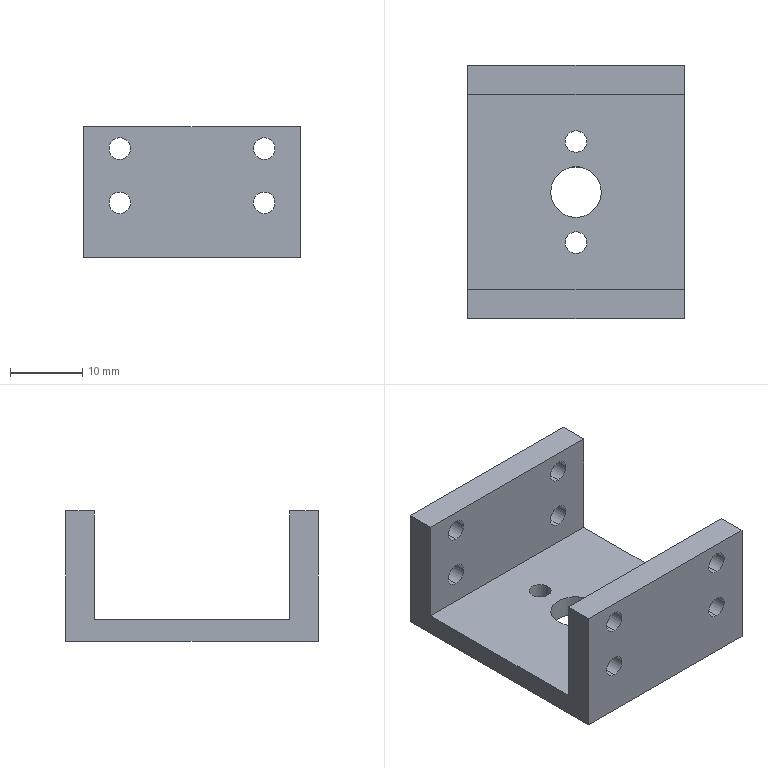Part | SolidWorks | features ICE 2, Extrusion 1, MirrorPattern 1 | 1 solid | 32 faces | box 30 x 35 x 18 mm | volume 6366 mm3 | cylinder 22 | plane 10 | commonest cylinder face diameters 3 x20 7 x2
STEP:
#1=CARTESIAN_POINT('',(-10.,-17.5,9.));
#2=VERTEX_POINT('',#1);
#3=CARTESIAN_POINT('',(-10.,-17.5,6.));
#4=VERTEX_POINT('',#3);
#5=CARTESIAN_POINT('',(-10.,-17.5,7.5));
#6=DIRECTION('',(0.,-1.,0.));
#7=DIRECTION('',(0.,0.,1.));
#8=AXIS2_PLACEMENT_3D('',#5,#6,#7);
#9=CIRCLE('',#8,1.5);
#10=EDGE_CURVE('',#2,#4,#9,.T.);
#11=ORIENTED_EDGE('',*,*,#10,.T.);
#12=CARTESIAN_POINT('',(-10.,-13.5,6.));
#13=VERTEX_POINT('',#12);
#14=CARTESIAN_POINT('',(-10.,-28.5,6.));
#15=DIRECTION('',(0.,1.,0.));
#16=VECTOR('',#15,1000.);
#17=LINE('',#14,#16);
#18=EDGE_CURVE('',#4,#13,#17,.T.);
#19=ORIENTED_EDGE('',*,*,#18,.T.);
#20=CARTESIAN_POINT('',(-10.,-13.5,9.));
#21=VERTEX_POINT('',#20);
#22=CARTESIAN_POINT('',(-10.,-13.5,7.5));
#23=DIRECTION('',(0.,-1.,0.));
#24=DIRECTION('',(0.,0.,1.));
#25=AXIS2_PLACEMENT_3D('',#22,#23,#24);
#26=CIRCLE('',#25,1.5);
#27=EDGE_CURVE('',#21,#13,#26,.T.);
#28=ORIENTED_EDGE('',*,*,#27,.F.);
#29=CARTESIAN_POINT('',(-10.,-28.5,9.));
#30=DIRECTION('',(0.,1.,0.));
#31=VECTOR('',#30,1000.);
#32=LINE('',#29,#31);
#33=EDGE_CURVE('',#2,#21,#32,.T.);
#34=ORIENTED_EDGE('',*,*,#33,.F.);
#35=EDGE_LOOP('',(#11,#19,#28,#34));
#36=FACE_OUTER_BOUND('',#35,.T.);
#37=CARTESIAN_POINT('',(-10.,-28.5,7.5));
#38=DIRECTION('',(0.,1.,0.));
#39=DIRECTION('',(0.,0.,1.));
#40=AXIS2_PLACEMENT_3D('',#37,#38,#39);
#41=CYLINDRICAL_SURFACE('',#40,1.5);
#42=ADVANCED_FACE('',(#36),#41,.F.);
#43=CARTESIAN_POINT('',(10.,-17.5,9.));
#44=VERTEX_POINT('',#43);
#45=CARTESIAN_POINT('',(10.,-17.5,6.));
#46=VERTEX_POINT('',#45);
#47=CARTESIAN_POINT('',(10.,-17.5,7.5));
#48=DIRECTION('',(0.,-1.,0.));
#49=DIRECTION('',(0.,0.,1.));
#50=AXIS2_PLACEMENT_3D('',#47,#48,#49);
#51=CIRCLE('',#50,1.5);
#52=EDGE_CURVE('',#44,#46,#51,.T.);
#53=ORIENTED_EDGE('',*,*,#52,.T.);
#54=CARTESIAN_POINT('',(10.,-13.5,6.));
#55=VERTEX_POINT('',#54);
#56=CARTESIAN_POINT('',(10.,-28.5,6.));
#57=DIRECTION('',(0.,1.,0.));
#58=VECTOR('',#57,1000.);
#59=LINE('',#56,#58);
#60=EDGE_CURVE('',#46,#55,#59,.T.);
#61=ORIENTED_EDGE('',*,*,#60,.T.);
#62=CARTESIAN_POINT('',(10.,-13.5,9.));
#63=VERTEX_POINT('',#62);
#64=CARTESIAN_POINT('',(10.,-13.5,7.5));
#65=DIRECTION('',(0.,-1.,0.));
#66=DIRECTION('',(0.,0.,-1.));
#67=AXIS2_PLACEMENT_3D('',#64,#65,#66);
#68=CIRCLE('',#67,1.5);
#69=EDGE_CURVE('',#63,#55,#68,.T.);
#70=ORIENTED_EDGE('',*,*,#69,.F.);
#71=CARTESIAN_POINT('',(10.,-28.5,9.));
#72=DIRECTION('',(0.,1.,0.));
#73=VECTOR('',#72,1000.);
#74=LINE('',#71,#73);
#75=EDGE_CURVE('',#44,#63,#74,.T.);
#76=ORIENTED_EDGE('',*,*,#75,.F.);
#77=EDGE_LOOP('',(#53,#61,#70,#76));
#78=FACE_OUTER_BOUND('',#77,.T.);
#79=CARTESIAN_POINT('',(10.,-28.5,7.5));
#80=DIRECTION('',(0.,1.,0.));
#81=DIRECTION('',(0.,0.,1.));
#82=AXIS2_PLACEMENT_3D('',#79,#80,#81);
#83=CYLINDRICAL_SURFACE('',#82,1.5);
#84=ADVANCED_FACE('',(#78),#83,.F.);
#85=CARTESIAN_POINT('',(10.,-17.5,16.5));
#86=VERTEX_POINT('',#85);
#87=CARTESIAN_POINT('',(10.,-17.5,13.5));
#88=VERTEX_POINT('',#87);
#89=CARTESIAN_POINT('',(10.,-17.5,15.));
#90=DIRECTION('',(0.,-1.,0.));
#91=DIRECTION('',(0.,0.,1.));
#92=AXIS2_PLACEMENT_3D('',#89,#90,#91);
#93=CIRCLE('',#92,1.5);
#94=EDGE_CURVE('',#86,#88,#93,.T.);
#95=ORIENTED_EDGE('',*,*,#94,.T.);
#96=CARTESIAN_POINT('',(10.,-13.5,13.5));
#97=VERTEX_POINT('',#96);
#98=CARTESIAN_POINT('',(10.,-28.5,13.5));
#99=DIRECTION('',(0.,1.,0.));
#100=VECTOR('',#99,1000.);
#101=LINE('',#98,#100);
#102=EDGE_CURVE('',#88,#97,#101,.T.);
#103=ORIENTED_EDGE('',*,*,#102,.T.);
#104=CARTESIAN_POINT('',(10.,-13.5,16.5));
#105=VERTEX_POINT('',#104);
#106=CARTESIAN_POINT('',(10.,-13.5,15.));
#107=DIRECTION('',(0.,-1.,0.));
#108=DIRECTION('',(0.,0.,1.));
#109=AXIS2_PLACEMENT_3D('',#106,#107,#108);
#110=CIRCLE('',#109,1.5);
#111=EDGE_CURVE('',#105,#97,#110,.T.);
#112=ORIENTED_EDGE('',*,*,#111,.F.);
#113=CARTESIAN_POINT('',(10.,-28.5,16.5));
#114=DIRECTION('',(0.,1.,0.));
#115=VECTOR('',#114,1000.);
#116=LINE('',#113,#115);
#117=EDGE_CURVE('',#86,#105,#116,.T.);
#118=ORIENTED_EDGE('',*,*,#117,.F.);
#119=EDGE_LOOP('',(#95,#103,#112,#118));
#120=FACE_OUTER_BOUND('',#119,.T.);
#121=CARTESIAN_POINT('',(10.,-28.5,15.));
#122=DIRECTION('',(0.,1.,0.));
#123=DIRECTION('',(0.,0.,1.));
#124=AXIS2_PLACEMENT_3D('',#121,#122,#123);
#125=CYLINDRICAL_SURFACE('',#124,1.5);
#126=ADVANCED_FACE('',(#120),#125,.F.);
#127=CARTESIAN_POINT('',(-10.,-17.5,16.5));
#128=VERTEX_POINT('',#127);
#129=CARTESIAN_POINT('',(-10.,-17.5,13.5));
#130=VERTEX_POINT('',#129);
#131=CARTESIAN_POINT('',(-10.,-17.5,15.));
#132=DIRECTION('',(0.,-1.,0.));
#133=DIRECTION('',(0.,0.,1.));
#134=AXIS2_PLACEMENT_3D('',#131,#132,#133);
#135=CIRCLE('',#134,1.5);
#136=EDGE_CURVE('',#128,#130,#135,.T.);
#137=ORIENTED_EDGE('',*,*,#136,.T.);
#138=CARTESIAN_POINT('',(-10.,-13.5,13.5));
#139=VERTEX_POINT('',#138);
#140=CARTESIAN_POINT('',(-10.,-28.5,13.5));
#141=DIRECTION('',(0.,1.,0.));
#142=VECTOR('',#141,1000.);
#143=LINE('',#140,#142);
#144=EDGE_CURVE('',#130,#139,#143,.T.);
#145=ORIENTED_EDGE('',*,*,#144,.T.);
#146=CARTESIAN_POINT('',(-10.,-13.5,16.5));
#147=VERTEX_POINT('',#146);
#148=CARTESIAN_POINT('',(-10.,-13.5,15.));
#149=DIRECTION('',(0.,-1.,0.));
#150=DIRECTION('',(0.,0.,-1.));
#151=AXIS2_PLACEMENT_3D('',#148,#149,#150);
#152=CIRCLE('',#151,1.5);
#153=EDGE_CURVE('',#147,#139,#152,.T.);
#154=ORIENTED_EDGE('',*,*,#153,.F.);
#155=CARTESIAN_POINT('',(-10.,-28.5,16.5));
#156=DIRECTION('',(0.,1.,0.));
#157=VECTOR('',#156,1000.);
#158=LINE('',#155,#157);
#159=EDGE_CURVE('',#128,#147,#158,.T.);
#160=ORIENTED_EDGE('',*,*,#159,.F.);
#161=EDGE_LOOP('',(#137,#145,#154,#160));
#162=FACE_OUTER_BOUND('',#161,.T.);
#163=CARTESIAN_POINT('',(-10.,-28.5,15.));
#164=DIRECTION('',(0.,1.,0.));
#165=DIRECTION('',(0.,0.,1.));
#166=AXIS2_PLACEMENT_3D('',#163,#164,#165);
#167=CYLINDRICAL_SURFACE('',#166,1.5);
#168=ADVANCED_FACE('',(#162),#167,.F.);
#169=CARTESIAN_POINT('',(-10.,17.5,9.));
#170=VERTEX_POINT('',#169);
#171=CARTESIAN_POINT('',(-10.,17.5,6.));
#172=VERTEX_POINT('',#171);
#173=CARTESIAN_POINT('',(-10.,17.5,7.5));
#174=DIRECTION('',(0.,-1.,0.));
#175=DIRECTION('',(0.,0.,-1.));
#176=AXIS2_PLACEMENT_3D('',#173,#174,#175);
#177=CIRCLE('',#176,1.5);
#178=EDGE_CURVE('',#170,#172,#177,.T.);
#179=ORIENTED_EDGE('',*,*,#178,.F.);
#180=CARTESIAN_POINT('',(-10.,13.5,9.));
#181=VERTEX_POINT('',#180);
#182=CARTESIAN_POINT('',(-10.,28.5,9.));
#183=DIRECTION('',(0.,-1.,0.));
#184=VECTOR('',#183,1000.);
#185=LINE('',#182,#184);
#186=EDGE_CURVE('',#170,#181,#185,.T.);
#187=ORIENTED_EDGE('',*,*,#186,.T.);
#188=CARTESIAN_POINT('',(-10.,13.5,6.));
#189=VERTEX_POINT('',#188);
#190=CARTESIAN_POINT('',(-10.,13.5,7.5));
#191=DIRECTION('',(0.,-1.,0.));
#192=DIRECTION('',(0.,0.,1.));
#193=AXIS2_PLACEMENT_3D('',#190,#191,#192);
#194=CIRCLE('',#193,1.5);
#195=EDGE_CURVE('',#181,#189,#194,.T.);
#196=ORIENTED_EDGE('',*,*,#195,.T.);
#197=CARTESIAN_POINT('',(-10.,28.5,6.));
#198=DIRECTION('',(0.,-1.,0.));
#199=VECTOR('',#198,1000.);
#200=LINE('',#197,#199);
#201=EDGE_CURVE('',#172,#189,#200,.T.);
#202=ORIENTED_EDGE('',*,*,#201,.F.);
#203=EDGE_LOOP('',(#179,#187,#196,#202));
#204=FACE_OUTER_BOUND('',#203,.T.);
#205=CARTESIAN_POINT('',(-10.,28.5,7.5));
#206=DIRECTION('',(0.,-1.,0.));
#207=DIRECTION('',(0.,0.,-1.));
#208=AXIS2_PLACEMENT_3D('',#205,#206,#207);
#209=CYLINDRICAL_SURFACE('',#208,1.5);
#210=ADVANCED_FACE('',(#204),#209,.F.);
#211=CARTESIAN_POINT('',(10.,17.5,9.));
#212=VERTEX_POINT('',#211);
#213=CARTESIAN_POINT('',(10.,17.5,6.));
#214=VERTEX_POINT('',#213);
#215=CARTESIAN_POINT('',(10.,17.5,7.5));
#216=DIRECTION('',(0.,-1.,0.));
#217=DIRECTION('',(0.,0.,-1.));
#218=AXIS2_PLACEMENT_3D('',#215,#216,#217);
#219=CIRCLE('',#218,1.5);
#220=EDGE_CURVE('',#212,#214,#219,.T.);
#221=ORIENTED_EDGE('',*,*,#220,.F.);
#222=CARTESIAN_POINT('',(10.,13.5,9.));
#223=VERTEX_POINT('',#222);
#224=CARTESIAN_POINT('',(10.,28.5,9.));
#225=DIRECTION('',(0.,-1.,0.));
#226=VECTOR('',#225,1000.);
#227=LINE('',#224,#226);
#228=EDGE_CURVE('',#212,#223,#227,.T.);
#229=ORIENTED_EDGE('',*,*,#228,.T.);
#230=CARTESIAN_POINT('',(10.,13.5,6.));
#231=VERTEX_POINT('',#230);
#232=CARTESIAN_POINT('',(10.,13.5,7.5));
#233=DIRECTION('',(0.,-1.,0.));
#234=DIRECTION('',(0.,0.,-1.));
#235=AXIS2_PLACEMENT_3D('',#232,#233,#234);
#236=CIRCLE('',#235,1.5);
#237=EDGE_CURVE('',#223,#231,#236,.T.);
#238=ORIENTED_EDGE('',*,*,#237,.T.);
#239=CARTESIAN_POINT('',(10.,28.5,6.));
#240=DIRECTION('',(0.,-1.,0.));
#241=VECTOR('',#240,1000.);
#242=LINE('',#239,#241);
#243=EDGE_CURVE('',#214,#231,#242,.T.);
#244=ORIENTED_EDGE('',*,*,#243,.F.);
#245=EDGE_LOOP('',(#221,#229,#238,#244));
#246=FACE_OUTER_BOUND('',#245,.T.);
#247=CARTESIAN_POINT('',(10.,28.5,7.5));
#248=DIRECTION('',(0.,-1.,0.));
#249=DIRECTION('',(0.,0.,-1.));
#250=AXIS2_PLACEMENT_3D('',#247,#248,#249);
#251=CYLINDRICAL_SURFACE('',#250,1.5);
#252=ADVANCED_FACE('',(#246),#251,.F.);
#253=CARTESIAN_POINT('',(10.,17.5,16.5));
#254=VERTEX_POINT('',#253);
#255=CARTESIAN_POINT('',(10.,17.5,13.5));
#256=VERTEX_POINT('',#255);
#257=CARTESIAN_POINT('',(10.,17.5,15.));
#258=DIRECTION('',(0.,-1.,0.));
#259=DIRECTION('',(0.,0.,-1.));
#260=AXIS2_PLACEMENT_3D('',#257,#258,#259);
#261=CIRCLE('',#260,1.5);
#262=EDGE_CURVE('',#254,#256,#261,.T.);
#263=ORIENTED_EDGE('',*,*,#262,.F.);
#264=CARTESIAN_POINT('',(10.,13.5,16.5));
#265=VERTEX_POINT('',#264);
#266=CARTESIAN_POINT('',(10.,28.5,16.5));
#267=DIRECTION('',(0.,-1.,0.));
#268=VECTOR('',#267,1000.);
#269=LINE('',#266,#268);
#270=EDGE_CURVE('',#254,#265,#269,.T.);
#271=ORIENTED_EDGE('',*,*,#270,.T.);
#272=CARTESIAN_POINT('',(10.,13.5,13.5));
#273=VERTEX_POINT('',#272);
#274=CARTESIAN_POINT('',(10.,13.5,15.));
#275=DIRECTION('',(0.,-1.,0.));
#276=DIRECTION('',(0.,0.,1.));
#277=AXIS2_PLACEMENT_3D('',#274,#275,#276);
#278=CIRCLE('',#277,1.5);
#279=EDGE_CURVE('',#265,#273,#278,.T.);
#280=ORIENTED_EDGE('',*,*,#279,.T.);
#281=CARTESIAN_POINT('',(10.,28.5,13.5));
#282=DIRECTION('',(0.,-1.,0.));
#283=VECTOR('',#282,1000.);
#284=LINE('',#281,#283);
#285=EDGE_CURVE('',#256,#273,#284,.T.);
#286=ORIENTED_EDGE('',*,*,#285,.F.);
#287=EDGE_LOOP('',(#263,#271,#280,#286));
#288=FACE_OUTER_BOUND('',#287,.T.);
#289=CARTESIAN_POINT('',(10.,28.5,15.));
#290=DIRECTION('',(0.,-1.,0.));
#291=DIRECTION('',(0.,0.,-1.));
#292=AXIS2_PLACEMENT_3D('',#289,#290,#291);
#293=CYLINDRICAL_SURFACE('',#292,1.5);
#294=ADVANCED_FACE('',(#288),#293,.F.);
#295=CARTESIAN_POINT('',(-10.,17.5,16.5));
#296=VERTEX_POINT('',#295);
#297=CARTESIAN_POINT('',(-10.,17.5,13.5));
#298=VERTEX_POINT('',#297);
#299=CARTESIAN_POINT('',(-10.,17.5,15.));
#300=DIRECTION('',(0.,-1.,0.));
#301=DIRECTION('',(0.,0.,-1.));
#302=AXIS2_PLACEMENT_3D('',#299,#300,#301);
#303=CIRCLE('',#302,1.5);
#304=EDGE_CURVE('',#296,#298,#303,.T.);
#305=ORIENTED_EDGE('',*,*,#304,.F.);
#306=CARTESIAN_POINT('',(-10.,13.5,16.5));
#307=VERTEX_POINT('',#306);
#308=CARTESIAN_POINT('',(-10.,28.5,16.5));
#309=DIRECTION('',(0.,-1.,0.));
#310=VECTOR('',#309,1000.);
#311=LINE('',#308,#310);
#312=EDGE_CURVE('',#296,#307,#311,.T.);
#313=ORIENTED_EDGE('',*,*,#312,.T.);
#314=CARTESIAN_POINT('',(-10.,13.5,13.5));
#315=VERTEX_POINT('',#314);
#316=CARTESIAN_POINT('',(-10.,13.5,15.));
#317=DIRECTION('',(0.,-1.,0.));
#318=DIRECTION('',(0.,0.,-1.));
#319=AXIS2_PLACEMENT_3D('',#316,#317,#318);
#320=CIRCLE('',#319,1.5);
#321=EDGE_CURVE('',#307,#315,#320,.T.);
#322=ORIENTED_EDGE('',*,*,#321,.T.);
#323=CARTESIAN_POINT('',(-10.,28.5,13.5));
#324=DIRECTION('',(0.,-1.,0.));
#325=VECTOR('',#324,1000.);
#326=LINE('',#323,#325);
#327=EDGE_CURVE('',#298,#315,#326,.T.);
#328=ORIENTED_EDGE('',*,*,#327,.F.);
#329=EDGE_LOOP('',(#305,#313,#322,#328));
#330=FACE_OUTER_BOUND('',#329,.T.);
#331=CARTESIAN_POINT('',(-10.,28.5,15.));
#332=DIRECTION('',(0.,-1.,0.));
#333=DIRECTION('',(0.,0.,-1.));
#334=AXIS2_PLACEMENT_3D('',#331,#332,#333);
#335=CYLINDRICAL_SURFACE('',#334,1.5);
#336=ADVANCED_FACE('',(#330),#335,.F.);
#337=CARTESIAN_POINT('',(-1.5,-7.,3.));
#338=VERTEX_POINT('',#337);
#339=CARTESIAN_POINT('',(1.5,-7.,3.));
#340=VERTEX_POINT('',#339);
#341=CARTESIAN_POINT('',(0.,-7.,3.));
#342=DIRECTION('',(0.,0.,1.));
#343=DIRECTION('',(-1.,0.,0.));
#344=AXIS2_PLACEMENT_3D('',#341,#342,#343);
#345=CIRCLE('',#344,1.5);
#346=EDGE_CURVE('',#338,#340,#345,.T.);
#347=ORIENTED_EDGE('',*,*,#346,.T.);
#348=CARTESIAN_POINT('',(1.5,-7.,0.));
#349=VERTEX_POINT('',#348);
#350=CARTESIAN_POINT('',(1.5,-7.,3.));
#351=DIRECTION('',(0.,0.,-1.));
#352=VECTOR('',#351,1000.);
#353=LINE('',#350,#352);
#354=EDGE_CURVE('',#340,#349,#353,.T.);
#355=ORIENTED_EDGE('',*,*,#354,.T.);
#356=CARTESIAN_POINT('',(-1.5,-7.,0.));
#357=VERTEX_POINT('',#356);
#358=CARTESIAN_POINT('',(0.,-7.,0.));
#359=DIRECTION('',(0.,0.,1.));
#360=DIRECTION('',(-1.,0.,0.));
#361=AXIS2_PLACEMENT_3D('',#358,#359,#360);
#362=CIRCLE('',#361,1.5);
#363=EDGE_CURVE('',#357,#349,#362,.T.);
#364=ORIENTED_EDGE('',*,*,#363,.F.);
#365=CARTESIAN_POINT('',(-1.5,-7.,3.));
#366=DIRECTION('',(0.,0.,-1.));
#367=VECTOR('',#366,1000.);
#368=LINE('',#365,#367);
#369=EDGE_CURVE('',#338,#357,#368,.T.);
#370=ORIENTED_EDGE('',*,*,#369,.F.);
#371=EDGE_LOOP('',(#347,#355,#364,#370));
#372=FACE_OUTER_BOUND('',#371,.T.);
#373=CARTESIAN_POINT('',(0.,-7.,3.));
#374=DIRECTION('',(0.,0.,-1.));
#375=DIRECTION('',(-1.,0.,0.));
#376=AXIS2_PLACEMENT_3D('',#373,#374,#375);
#377=CYLINDRICAL_SURFACE('',#376,1.5);
#378=ADVANCED_FACE('',(#372),#377,.F.);
#379=CARTESIAN_POINT('',(-1.5,7.,3.));
#380=VERTEX_POINT('',#379);
#381=CARTESIAN_POINT('',(1.5,7.,3.));
#382=VERTEX_POINT('',#381);
#383=CARTESIAN_POINT('',(0.,7.,3.));
#384=DIRECTION('',(0.,0.,1.));
#385=DIRECTION('',(1.,0.,0.));
#386=AXIS2_PLACEMENT_3D('',#383,#384,#385);
#387=CIRCLE('',#386,1.5);
#388=EDGE_CURVE('',#380,#382,#387,.T.);
#389=ORIENTED_EDGE('',*,*,#388,.T.);
#390=CARTESIAN_POINT('',(1.5,7.,0.));
#391=VERTEX_POINT('',#390);
#392=CARTESIAN_POINT('',(1.5,7.,3.));
#393=DIRECTION('',(0.,0.,-1.));
#394=VECTOR('',#393,1000.);
#395=LINE('',#392,#394);
#396=EDGE_CURVE('',#382,#391,#395,.T.);
#397=ORIENTED_EDGE('',*,*,#396,.T.);
#398=CARTESIAN_POINT('',(-1.5,7.,0.));
#399=VERTEX_POINT('',#398);
#400=CARTESIAN_POINT('',(0.,7.,0.));
#401=DIRECTION('',(0.,0.,1.));
#402=DIRECTION('',(1.,0.,0.));
#403=AXIS2_PLACEMENT_3D('',#400,#401,#402);
#404=CIRCLE('',#403,1.5);
#405=EDGE_CURVE('',#399,#391,#404,.T.);
#406=ORIENTED_EDGE('',*,*,#405,.F.);
#407=CARTESIAN_POINT('',(-1.5,7.,3.));
#408=DIRECTION('',(0.,0.,-1.));
#409=VECTOR('',#408,1000.);
#410=LINE('',#407,#409);
#411=EDGE_CURVE('',#380,#399,#410,.T.);
#412=ORIENTED_EDGE('',*,*,#411,.F.);
#413=EDGE_LOOP('',(#389,#397,#406,#412));
#414=FACE_OUTER_BOUND('',#413,.T.);
#415=CARTESIAN_POINT('',(0.,7.,3.));
#416=DIRECTION('',(0.,0.,-1.));
#417=DIRECTION('',(-1.,0.,0.));
#418=AXIS2_PLACEMENT_3D('',#415,#416,#417);
#419=CYLINDRICAL_SURFACE('',#418,1.5);
#420=ADVANCED_FACE('',(#414),#419,.F.);
#421=CARTESIAN_POINT('',(-3.5,0.,3.));
#422=VERTEX_POINT('',#421);
#423=CARTESIAN_POINT('',(3.5,0.,3.));
#424=VERTEX_POINT('',#423);
#425=CARTESIAN_POINT('',(0.,0.,3.));
#426=DIRECTION('',(0.,0.,1.));
#427=DIRECTION('',(1.,0.,0.));
#428=AXIS2_PLACEMENT_3D('',#425,#426,#427);
#429=CIRCLE('',#428,3.5);
#430=EDGE_CURVE('',#422,#424,#429,.T.);
#431=ORIENTED_EDGE('',*,*,#430,.T.);
#432=CARTESIAN_POINT('',(3.5,0.,0.));
#433=VERTEX_POINT('',#432);
#434=CARTESIAN_POINT('',(3.5,0.,3.));
#435=DIRECTION('',(0.,0.,-1.));
#436=VECTOR('',#435,1000.);
#437=LINE('',#434,#436);
#438=EDGE_CURVE('',#424,#433,#437,.T.);
#439=ORIENTED_EDGE('',*,*,#438,.T.);
#440=CARTESIAN_POINT('',(-3.5,0.,0.));
#441=VERTEX_POINT('',#440);
#442=CARTESIAN_POINT('',(0.,0.,0.));
#443=DIRECTION('',(0.,0.,1.));
#444=DIRECTION('',(1.,0.,0.));
#445=AXIS2_PLACEMENT_3D('',#442,#443,#444);
#446=CIRCLE('',#445,3.5);
#447=EDGE_CURVE('',#441,#433,#446,.T.);
#448=ORIENTED_EDGE('',*,*,#447,.F.);
#449=CARTESIAN_POINT('',(-3.5,0.,3.));
#450=DIRECTION('',(0.,0.,-1.));
#451=VECTOR('',#450,1000.);
#452=LINE('',#449,#451);
#453=EDGE_CURVE('',#422,#441,#452,.T.);
#454=ORIENTED_EDGE('',*,*,#453,.F.);
#455=EDGE_LOOP('',(#431,#439,#448,#454));
#456=FACE_OUTER_BOUND('',#455,.T.);
#457=CARTESIAN_POINT('',(0.,0.,3.));
#458=DIRECTION('',(0.,0.,-1.));
#459=DIRECTION('',(-1.,0.,0.));
#460=AXIS2_PLACEMENT_3D('',#457,#458,#459);
#461=CYLINDRICAL_SURFACE('',#460,3.5);
#462=ADVANCED_FACE('',(#456),#461,.F.);
#463=ORIENTED_EDGE('',*,*,#430,.F.);
#464=CARTESIAN_POINT('',(0.,0.,3.));
#465=DIRECTION('',(0.,0.,1.));
#466=DIRECTION('',(1.,0.,0.));
#467=AXIS2_PLACEMENT_3D('',#464,#465,#466);
#468=CIRCLE('',#467,3.5);
#469=EDGE_CURVE('',#424,#422,#468,.T.);
#470=ORIENTED_EDGE('',*,*,#469,.F.);
#471=EDGE_LOOP('',(#463,#470));
#472=FACE_BOUND('',#471,.T.);
#473=ORIENTED_EDGE('',*,*,#388,.F.);
#474=CARTESIAN_POINT('',(0.,7.,3.));
#475=DIRECTION('',(0.,0.,1.));
#476=DIRECTION('',(1.,0.,0.));
#477=AXIS2_PLACEMENT_3D('',#474,#475,#476);
#478=CIRCLE('',#477,1.5);
#479=EDGE_CURVE('',#382,#380,#478,.T.);
#480=ORIENTED_EDGE('',*,*,#479,.F.);
#481=EDGE_LOOP('',(#473,#480));
#482=FACE_BOUND('',#481,.T.);
#483=ORIENTED_EDGE('',*,*,#346,.F.);
#484=CARTESIAN_POINT('',(0.,-7.,3.));
#485=DIRECTION('',(0.,0.,1.));
#486=DIRECTION('',(-1.,0.,0.));
#487=AXIS2_PLACEMENT_3D('',#484,#485,#486);
#488=CIRCLE('',#487,1.5);
#489=EDGE_CURVE('',#340,#338,#488,.T.);
#490=ORIENTED_EDGE('',*,*,#489,.F.);
#491=EDGE_LOOP('',(#483,#490));
#492=FACE_BOUND('',#491,.T.);
#493=CARTESIAN_POINT('',(15.,-13.5,3.));
#494=VERTEX_POINT('',#493);
#495=CARTESIAN_POINT('',(-15.,-13.5,3.));
#496=VERTEX_POINT('',#495);
#497=CARTESIAN_POINT('',(-15.,-13.5,3.));
#498=DIRECTION('',(-1.,0.,0.));
#499=VECTOR('',#498,1000.);
#500=LINE('',#497,#499);
#501=EDGE_CURVE('',#494,#496,#500,.T.);
#502=ORIENTED_EDGE('',*,*,#501,.F.);
#503=CARTESIAN_POINT('',(15.,13.5,3.));
#504=VERTEX_POINT('',#503);
#505=CARTESIAN_POINT('',(15.,-17.5,3.));
#506=DIRECTION('',(0.,1.,0.));
#507=VECTOR('',#506,1000.);
#508=LINE('',#505,#507);
#509=EDGE_CURVE('',#494,#504,#508,.T.);
#510=ORIENTED_EDGE('',*,*,#509,.T.);
#511=CARTESIAN_POINT('',(-15.,13.5,3.));
#512=VERTEX_POINT('',#511);
#513=CARTESIAN_POINT('',(-15.,13.5,3.));
#514=DIRECTION('',(1.,0.,0.));
#515=VECTOR('',#514,1000.);
#516=LINE('',#513,#515);
#517=EDGE_CURVE('',#512,#504,#516,.T.);
#518=ORIENTED_EDGE('',*,*,#517,.F.);
#519=CARTESIAN_POINT('',(-15.,-17.5,3.));
#520=DIRECTION('',(0.,-1.,0.));
#521=VECTOR('',#520,1000.);
#522=LINE('',#519,#521);
#523=EDGE_CURVE('',#512,#496,#522,.T.);
#524=ORIENTED_EDGE('',*,*,#523,.T.);
#525=EDGE_LOOP('',(#502,#510,#518,#524));
#526=FACE_OUTER_BOUND('',#525,.T.);
#527=CARTESIAN_POINT('',(0.,0.,3.));
#528=DIRECTION('',(0.,0.,-1.));
#529=DIRECTION('',(-1.,0.,0.));
#530=AXIS2_PLACEMENT_3D('',#527,#528,#529);
#531=PLANE('',#530);
#532=ADVANCED_FACE('',(#472,#482,#492,#526),#531,.F.);
#533=ORIENTED_EDGE('',*,*,#405,.T.);
#534=CARTESIAN_POINT('',(0.,7.,0.));
#535=DIRECTION('',(0.,0.,1.));
#536=DIRECTION('',(1.,0.,0.));
#537=AXIS2_PLACEMENT_3D('',#534,#535,#536);
#538=CIRCLE('',#537,1.5);
#539=EDGE_CURVE('',#391,#399,#538,.T.);
#540=ORIENTED_EDGE('',*,*,#539,.T.);
#541=EDGE_LOOP('',(#533,#540));
#542=FACE_BOUND('',#541,.T.);
#543=CARTESIAN_POINT('',(15.,-17.5,0.));
#544=VERTEX_POINT('',#543);
#545=CARTESIAN_POINT('',(15.,17.5,0.));
#546=VERTEX_POINT('',#545);
#547=CARTESIAN_POINT('',(15.,-17.5,0.));
#548=DIRECTION('',(0.,1.,0.));
#549=VECTOR('',#548,1000.);
#550=LINE('',#547,#549);
#551=EDGE_CURVE('',#544,#546,#550,.T.);
#552=ORIENTED_EDGE('',*,*,#551,.F.);
#553=CARTESIAN_POINT('',(-15.,-17.5,0.));
#554=VERTEX_POINT('',#553);
#555=CARTESIAN_POINT('',(-15.,-17.5,0.));
#556=DIRECTION('',(1.,0.,0.));
#557=VECTOR('',#556,1000.);
#558=LINE('',#555,#557);
#559=EDGE_CURVE('',#554,#544,#558,.T.);
#560=ORIENTED_EDGE('',*,*,#559,.F.);
#561=CARTESIAN_POINT('',(-15.,17.5,0.));
#562=VERTEX_POINT('',#561);
#563=CARTESIAN_POINT('',(-15.,-17.5,0.));
#564=DIRECTION('',(0.,-1.,0.));
#565=VECTOR('',#564,1000.);
#566=LINE('',#563,#565);
#567=EDGE_CURVE('',#562,#554,#566,.T.);
#568=ORIENTED_EDGE('',*,*,#567,.F.);
#569=CARTESIAN_POINT('',(-15.,17.5,0.));
#570=DIRECTION('',(-1.,0.,0.));
#571=VECTOR('',#570,1000.);
#572=LINE('',#569,#571);
#573=EDGE_CURVE('',#546,#562,#572,.T.);
#574=ORIENTED_EDGE('',*,*,#573,.F.);
#575=EDGE_LOOP('',(#552,#560,#568,#574));
#576=FACE_OUTER_BOUND('',#575,.T.);
#577=ORIENTED_EDGE('',*,*,#447,.T.);
#578=CARTESIAN_POINT('',(0.,0.,0.));
#579=DIRECTION('',(0.,0.,1.));
#580=DIRECTION('',(1.,0.,0.));
#581=AXIS2_PLACEMENT_3D('',#578,#579,#580);
#582=CIRCLE('',#581,3.5);
#583=EDGE_CURVE('',#433,#441,#582,.T.);
#584=ORIENTED_EDGE('',*,*,#583,.T.);
#585=EDGE_LOOP('',(#577,#584));
#586=FACE_BOUND('',#585,.T.);
#587=ORIENTED_EDGE('',*,*,#363,.T.);
#588=CARTESIAN_POINT('',(0.,-7.,0.));
#589=DIRECTION('',(0.,0.,1.));
#590=DIRECTION('',(-1.,0.,0.));
#591=AXIS2_PLACEMENT_3D('',#588,#589,#590);
#592=CIRCLE('',#591,1.5);
#593=EDGE_CURVE('',#349,#357,#592,.T.);
#594=ORIENTED_EDGE('',*,*,#593,.T.);
#595=EDGE_LOOP('',(#587,#594));
#596=FACE_BOUND('',#595,.T.);
#597=CARTESIAN_POINT('',(0.,0.,0.));
#598=DIRECTION('',(0.,0.,-1.));
#599=DIRECTION('',(-1.,0.,0.));
#600=AXIS2_PLACEMENT_3D('',#597,#598,#599);
#601=PLANE('',#600);
#602=ADVANCED_FACE('',(#542,#576,#586,#596),#601,.T.);
#603=ORIENTED_EDGE('',*,*,#551,.T.);
#604=CARTESIAN_POINT('',(15.,17.5,18.));
#605=VERTEX_POINT('',#604);
#606=CARTESIAN_POINT('',(15.,17.5,3.));
#607=DIRECTION('',(0.,0.,-1.));
#608=VECTOR('',#607,1000.);
#609=LINE('',#606,#608);
#610=EDGE_CURVE('',#605,#546,#609,.T.);
#611=ORIENTED_EDGE('',*,*,#610,.F.);
#612=CARTESIAN_POINT('',(15.,13.5,18.));
#613=VERTEX_POINT('',#612);
#614=CARTESIAN_POINT('',(15.,17.5,18.));
#615=DIRECTION('',(0.,1.,0.));
#616=VECTOR('',#615,1000.);
#617=LINE('',#614,#616);
#618=EDGE_CURVE('',#613,#605,#617,.T.);
#619=ORIENTED_EDGE('',*,*,#618,.F.);
#620=CARTESIAN_POINT('',(15.,13.5,18.));
#621=DIRECTION('',(0.,0.,-1.));
#622=VECTOR('',#621,1000.);
#623=LINE('',#620,#622);
#624=EDGE_CURVE('',#613,#504,#623,.T.);
#625=ORIENTED_EDGE('',*,*,#624,.T.);
#626=ORIENTED_EDGE('',*,*,#509,.F.);
#627=CARTESIAN_POINT('',(15.,-13.5,18.));
#628=VERTEX_POINT('',#627);
#629=CARTESIAN_POINT('',(15.,-13.5,18.));
#630=DIRECTION('',(0.,0.,-1.));
#631=VECTOR('',#630,1000.);
#632=LINE('',#629,#631);
#633=EDGE_CURVE('',#628,#494,#632,.T.);
#634=ORIENTED_EDGE('',*,*,#633,.F.);
#635=CARTESIAN_POINT('',(15.,-17.5,18.));
#636=VERTEX_POINT('',#635);
#637=CARTESIAN_POINT('',(15.,-17.5,18.));
#638=DIRECTION('',(0.,1.,0.));
#639=VECTOR('',#638,1000.);
#640=LINE('',#637,#639);
#641=EDGE_CURVE('',#636,#628,#640,.T.);
#642=ORIENTED_EDGE('',*,*,#641,.F.);
#643=CARTESIAN_POINT('',(15.,-17.5,3.));
#644=DIRECTION('',(0.,0.,-1.));
#645=VECTOR('',#644,1000.);
#646=LINE('',#643,#645);
#647=EDGE_CURVE('',#636,#544,#646,.T.);
#648=ORIENTED_EDGE('',*,*,#647,.T.);
#649=EDGE_LOOP('',(#603,#611,#619,#625,#626,#634,#642,#648));
#650=FACE_OUTER_BOUND('',#649,.T.);
#651=CARTESIAN_POINT('',(15.,-17.5,3.));
#652=DIRECTION('',(-1.,0.,0.));
#653=DIRECTION('',(0.,0.,1.));
#654=AXIS2_PLACEMENT_3D('',#651,#652,#653);
#655=PLANE('',#654);
#656=ADVANCED_FACE('',(#650),#655,.F.);
#657=CARTESIAN_POINT('',(-10.,17.5,7.5));
#658=DIRECTION('',(0.,-1.,0.));
#659=DIRECTION('',(0.,0.,-1.));
#660=AXIS2_PLACEMENT_3D('',#657,#658,#659);
#661=CIRCLE('',#660,1.5);
#662=EDGE_CURVE('',#172,#170,#661,.T.);
#663=ORIENTED_EDGE('',*,*,#662,.T.);
#664=ORIENTED_EDGE('',*,*,#178,.T.);
#665=EDGE_LOOP('',(#663,#664));
#666=FACE_BOUND('',#665,.T.);
#667=CARTESIAN_POINT('',(10.,17.5,7.5));
#668=DIRECTION('',(0.,-1.,0.));
#669=DIRECTION('',(0.,0.,-1.));
#670=AXIS2_PLACEMENT_3D('',#667,#668,#669);
#671=CIRCLE('',#670,1.5);
#672=EDGE_CURVE('',#214,#212,#671,.T.);
#673=ORIENTED_EDGE('',*,*,#672,.T.);
#674=ORIENTED_EDGE('',*,*,#220,.T.);
#675=EDGE_LOOP('',(#673,#674));
#676=FACE_BOUND('',#675,.T.);
#677=CARTESIAN_POINT('',(10.,17.5,15.));
#678=DIRECTION('',(0.,-1.,0.));
#679=DIRECTION('',(0.,0.,-1.));
#680=AXIS2_PLACEMENT_3D('',#677,#678,#679);
#681=CIRCLE('',#680,1.5);
#682=EDGE_CURVE('',#256,#254,#681,.T.);
#683=ORIENTED_EDGE('',*,*,#682,.T.);
#684=ORIENTED_EDGE('',*,*,#262,.T.);
#685=EDGE_LOOP('',(#683,#684));
#686=FACE_BOUND('',#685,.T.);
#687=CARTESIAN_POINT('',(-10.,17.5,15.));
#688=DIRECTION('',(0.,-1.,0.));
#689=DIRECTION('',(0.,0.,-1.));
#690=AXIS2_PLACEMENT_3D('',#687,#688,#689);
#691=CIRCLE('',#690,1.5);
#692=EDGE_CURVE('',#298,#296,#691,.T.);
#693=ORIENTED_EDGE('',*,*,#692,.T.);
#694=ORIENTED_EDGE('',*,*,#304,.T.);
#695=EDGE_LOOP('',(#693,#694));
#696=FACE_BOUND('',#695,.T.);
#697=ORIENTED_EDGE('',*,*,#573,.T.);
#698=CARTESIAN_POINT('',(-15.,17.5,18.));
#699=VERTEX_POINT('',#698);
#700=CARTESIAN_POINT('',(-15.,17.5,3.));
#701=DIRECTION('',(0.,0.,-1.));
#702=VECTOR('',#701,1000.);
#703=LINE('',#700,#702);
#704=EDGE_CURVE('',#699,#562,#703,.T.);
#705=ORIENTED_EDGE('',*,*,#704,.F.);
#706=CARTESIAN_POINT('',(-15.,17.5,18.));
#707=DIRECTION('',(-1.,0.,0.));
#708=VECTOR('',#707,1000.);
#709=LINE('',#706,#708);
#710=EDGE_CURVE('',#605,#699,#709,.T.);
#711=ORIENTED_EDGE('',*,*,#710,.F.);
#712=ORIENTED_EDGE('',*,*,#610,.T.);
#713=EDGE_LOOP('',(#697,#705,#711,#712));
#714=FACE_OUTER_BOUND('',#713,.T.);
#715=CARTESIAN_POINT('',(-15.,17.5,3.));
#716=DIRECTION('',(0.,-1.,0.));
#717=DIRECTION('',(0.,0.,-1.));
#718=AXIS2_PLACEMENT_3D('',#715,#716,#717);
#719=PLANE('',#718);
#720=ADVANCED_FACE('',(#666,#676,#686,#696,#714),#719,.F.);
#721=ORIENTED_EDGE('',*,*,#567,.T.);
#722=CARTESIAN_POINT('',(-15.,-17.5,18.));
#723=VERTEX_POINT('',#722);
#724=CARTESIAN_POINT('',(-15.,-17.5,3.));
#725=DIRECTION('',(0.,0.,-1.));
#726=VECTOR('',#725,1000.);
#727=LINE('',#724,#726);
#728=EDGE_CURVE('',#723,#554,#727,.T.);
#729=ORIENTED_EDGE('',*,*,#728,.F.);
#730=CARTESIAN_POINT('',(-15.,-13.5,18.));
#731=VERTEX_POINT('',#730);
#732=CARTESIAN_POINT('',(-15.,-17.5,18.));
#733=DIRECTION('',(0.,-1.,0.));
#734=VECTOR('',#733,1000.);
#735=LINE('',#732,#734);
#736=EDGE_CURVE('',#731,#723,#735,.T.);
#737=ORIENTED_EDGE('',*,*,#736,.F.);
#738=CARTESIAN_POINT('',(-15.,-13.5,18.));
#739=DIRECTION('',(0.,0.,-1.));
#740=VECTOR('',#739,1000.);
#741=LINE('',#738,#740);
#742=EDGE_CURVE('',#731,#496,#741,.T.);
#743=ORIENTED_EDGE('',*,*,#742,.T.);
#744=ORIENTED_EDGE('',*,*,#523,.F.);
#745=CARTESIAN_POINT('',(-15.,13.5,18.));
#746=VERTEX_POINT('',#745);
#747=CARTESIAN_POINT('',(-15.,13.5,18.));
#748=DIRECTION('',(0.,0.,-1.));
#749=VECTOR('',#748,1000.);
#750=LINE('',#747,#749);
#751=EDGE_CURVE('',#746,#512,#750,.T.);
#752=ORIENTED_EDGE('',*,*,#751,.F.);
#753=CARTESIAN_POINT('',(-15.,17.5,18.));
#754=DIRECTION('',(0.,-1.,0.));
#755=VECTOR('',#754,1000.);
#756=LINE('',#753,#755);
#757=EDGE_CURVE('',#699,#746,#756,.T.);
#758=ORIENTED_EDGE('',*,*,#757,.F.);
#759=ORIENTED_EDGE('',*,*,#704,.T.);
#760=EDGE_LOOP('',(#721,#729,#737,#743,#744,#752,#758,#759));
#761=FACE_OUTER_BOUND('',#760,.T.);
#762=CARTESIAN_POINT('',(-15.,-17.5,3.));
#763=DIRECTION('',(1.,0.,0.));
#764=DIRECTION('',(0.,0.,-1.));
#765=AXIS2_PLACEMENT_3D('',#762,#763,#764);
#766=PLANE('',#765);
#767=ADVANCED_FACE('',(#761),#766,.F.);
#768=ORIENTED_EDGE('',*,*,#10,.F.);
#769=CARTESIAN_POINT('',(-10.,-17.5,7.5));
#770=DIRECTION('',(0.,-1.,0.));
#771=DIRECTION('',(0.,0.,1.));
#772=AXIS2_PLACEMENT_3D('',#769,#770,#771);
#773=CIRCLE('',#772,1.5);
#774=EDGE_CURVE('',#4,#2,#773,.T.);
#775=ORIENTED_EDGE('',*,*,#774,.F.);
#776=EDGE_LOOP('',(#768,#775));
#777=FACE_BOUND('',#776,.T.);
#778=ORIENTED_EDGE('',*,*,#52,.F.);
#779=CARTESIAN_POINT('',(10.,-17.5,7.5));
#780=DIRECTION('',(0.,-1.,0.));
#781=DIRECTION('',(0.,0.,1.));
#782=AXIS2_PLACEMENT_3D('',#779,#780,#781);
#783=CIRCLE('',#782,1.5);
#784=EDGE_CURVE('',#46,#44,#783,.T.);
#785=ORIENTED_EDGE('',*,*,#784,.F.);
#786=EDGE_LOOP('',(#778,#785));
#787=FACE_BOUND('',#786,.T.);
#788=ORIENTED_EDGE('',*,*,#94,.F.);
#789=CARTESIAN_POINT('',(10.,-17.5,15.));
#790=DIRECTION('',(0.,-1.,0.));
#791=DIRECTION('',(0.,0.,1.));
#792=AXIS2_PLACEMENT_3D('',#789,#790,#791);
#793=CIRCLE('',#792,1.5);
#794=EDGE_CURVE('',#88,#86,#793,.T.);
#795=ORIENTED_EDGE('',*,*,#794,.F.);
#796=EDGE_LOOP('',(#788,#795));
#797=FACE_BOUND('',#796,.T.);
#798=ORIENTED_EDGE('',*,*,#136,.F.);
#799=CARTESIAN_POINT('',(-10.,-17.5,15.));
#800=DIRECTION('',(0.,-1.,0.));
#801=DIRECTION('',(0.,0.,1.));
#802=AXIS2_PLACEMENT_3D('',#799,#800,#801);
#803=CIRCLE('',#802,1.5);
#804=EDGE_CURVE('',#130,#128,#803,.T.);
#805=ORIENTED_EDGE('',*,*,#804,.F.);
#806=EDGE_LOOP('',(#798,#805));
#807=FACE_BOUND('',#806,.T.);
#808=ORIENTED_EDGE('',*,*,#559,.T.);
#809=ORIENTED_EDGE('',*,*,#647,.F.);
#810=CARTESIAN_POINT('',(-15.,-17.5,18.));
#811=DIRECTION('',(1.,0.,0.));
#812=VECTOR('',#811,1000.);
#813=LINE('',#810,#812);
#814=EDGE_CURVE('',#723,#636,#813,.T.);
#815=ORIENTED_EDGE('',*,*,#814,.F.);
#816=ORIENTED_EDGE('',*,*,#728,.T.);
#817=EDGE_LOOP('',(#808,#809,#815,#816));
#818=FACE_OUTER_BOUND('',#817,.T.);
#819=CARTESIAN_POINT('',(-15.,-17.5,3.));
#820=DIRECTION('',(0.,1.,0.));
#821=DIRECTION('',(0.,0.,1.));
#822=AXIS2_PLACEMENT_3D('',#819,#820,#821);
#823=PLANE('',#822);
#824=ADVANCED_FACE('',(#777,#787,#797,#807,#818),#823,.F.);
#825=ORIENTED_EDGE('',*,*,#438,.F.);
#826=ORIENTED_EDGE('',*,*,#469,.T.);
#827=ORIENTED_EDGE('',*,*,#453,.T.);
#828=ORIENTED_EDGE('',*,*,#583,.F.);
#829=EDGE_LOOP('',(#825,#826,#827,#828));
#830=FACE_OUTER_BOUND('',#829,.T.);
#831=CARTESIAN_POINT('',(0.,0.,3.));
#832=DIRECTION('',(0.,0.,-1.));
#833=DIRECTION('',(-1.,0.,0.));
#834=AXIS2_PLACEMENT_3D('',#831,#832,#833);
#835=CYLINDRICAL_SURFACE('',#834,3.5);
#836=ADVANCED_FACE('',(#830),#835,.F.);
#837=ORIENTED_EDGE('',*,*,#396,.F.);
#838=ORIENTED_EDGE('',*,*,#479,.T.);
#839=ORIENTED_EDGE('',*,*,#411,.T.);
#840=ORIENTED_EDGE('',*,*,#539,.F.);
#841=EDGE_LOOP('',(#837,#838,#839,#840));
#842=FACE_OUTER_BOUND('',#841,.T.);
#843=CARTESIAN_POINT('',(0.,7.,3.));
#844=DIRECTION('',(0.,0.,-1.));
#845=DIRECTION('',(-1.,0.,0.));
#846=AXIS2_PLACEMENT_3D('',#843,#844,#845);
#847=CYLINDRICAL_SURFACE('',#846,1.5);
#848=ADVANCED_FACE('',(#842),#847,.F.);
#849=ORIENTED_EDGE('',*,*,#354,.F.);
#850=ORIENTED_EDGE('',*,*,#489,.T.);
#851=ORIENTED_EDGE('',*,*,#369,.T.);
#852=ORIENTED_EDGE('',*,*,#593,.F.);
#853=EDGE_LOOP('',(#849,#850,#851,#852));
#854=FACE_OUTER_BOUND('',#853,.T.);
#855=CARTESIAN_POINT('',(0.,-7.,3.));
#856=DIRECTION('',(0.,0.,-1.));
#857=DIRECTION('',(-1.,0.,0.));
#858=AXIS2_PLACEMENT_3D('',#855,#856,#857);
#859=CYLINDRICAL_SURFACE('',#858,1.5);
#860=ADVANCED_FACE('',(#854),#859,.F.);
#861=CARTESIAN_POINT('',(-10.,13.5,7.5));
#862=DIRECTION('',(0.,-1.,0.));
#863=DIRECTION('',(0.,0.,1.));
#864=AXIS2_PLACEMENT_3D('',#861,#862,#863);
#865=CIRCLE('',#864,1.5);
#866=EDGE_CURVE('',#189,#181,#865,.T.);
#867=ORIENTED_EDGE('',*,*,#866,.F.);
#868=ORIENTED_EDGE('',*,*,#195,.F.);
#869=EDGE_LOOP('',(#867,#868));
#870=FACE_BOUND('',#869,.T.);
#871=CARTESIAN_POINT('',(10.,13.5,7.5));
#872=DIRECTION('',(0.,-1.,0.));
#873=DIRECTION('',(0.,0.,-1.));
#874=AXIS2_PLACEMENT_3D('',#871,#872,#873);
#875=CIRCLE('',#874,1.5);
#876=EDGE_CURVE('',#231,#223,#875,.T.);
#877=ORIENTED_EDGE('',*,*,#876,.F.);
#878=ORIENTED_EDGE('',*,*,#237,.F.);
#879=EDGE_LOOP('',(#877,#878));
#880=FACE_BOUND('',#879,.T.);
#881=CARTESIAN_POINT('',(10.,13.5,15.));
#882=DIRECTION('',(0.,-1.,0.));
#883=DIRECTION('',(0.,0.,1.));
#884=AXIS2_PLACEMENT_3D('',#881,#882,#883);
#885=CIRCLE('',#884,1.5);
#886=EDGE_CURVE('',#273,#265,#885,.T.);
#887=ORIENTED_EDGE('',*,*,#886,.F.);
#888=ORIENTED_EDGE('',*,*,#279,.F.);
#889=EDGE_LOOP('',(#887,#888));
#890=FACE_BOUND('',#889,.T.);
#891=CARTESIAN_POINT('',(-10.,13.5,15.));
#892=DIRECTION('',(0.,-1.,0.));
#893=DIRECTION('',(0.,0.,-1.));
#894=AXIS2_PLACEMENT_3D('',#891,#892,#893);
#895=CIRCLE('',#894,1.5);
#896=EDGE_CURVE('',#315,#307,#895,.T.);
#897=ORIENTED_EDGE('',*,*,#896,.F.);
#898=ORIENTED_EDGE('',*,*,#321,.F.);
#899=EDGE_LOOP('',(#897,#898));
#900=FACE_BOUND('',#899,.T.);
#901=ORIENTED_EDGE('',*,*,#517,.T.);
#902=ORIENTED_EDGE('',*,*,#624,.F.);
#903=CARTESIAN_POINT('',(-15.,13.5,18.));
#904=DIRECTION('',(1.,0.,0.));
#905=VECTOR('',#904,1000.);
#906=LINE('',#903,#905);
#907=EDGE_CURVE('',#746,#613,#906,.T.);
#908=ORIENTED_EDGE('',*,*,#907,.F.);
#909=ORIENTED_EDGE('',*,*,#751,.T.);
#910=EDGE_LOOP('',(#901,#902,#908,#909));
#911=FACE_OUTER_BOUND('',#910,.T.);
#912=CARTESIAN_POINT('',(-15.,13.5,18.));
#913=DIRECTION('',(0.,1.,0.));
#914=DIRECTION('',(0.,0.,1.));
#915=AXIS2_PLACEMENT_3D('',#912,#913,#914);
#916=PLANE('',#915);
#917=ADVANCED_FACE('',(#870,#880,#890,#900,#911),#916,.F.);
#918=ORIENTED_EDGE('',*,*,#757,.T.);
#919=ORIENTED_EDGE('',*,*,#907,.T.);
#920=ORIENTED_EDGE('',*,*,#618,.T.);
#921=ORIENTED_EDGE('',*,*,#710,.T.);
#922=EDGE_LOOP('',(#918,#919,#920,#921));
#923=FACE_OUTER_BOUND('',#922,.T.);
#924=CARTESIAN_POINT('',(0.,0.,18.));
#925=DIRECTION('',(0.,0.,1.));
#926=DIRECTION('',(1.,0.,0.));
#927=AXIS2_PLACEMENT_3D('',#924,#925,#926);
#928=PLANE('',#927);
#929=ADVANCED_FACE('',(#923),#928,.T.);
#930=ORIENTED_EDGE('',*,*,#27,.T.);
#931=CARTESIAN_POINT('',(-10.,-13.5,7.5));
#932=DIRECTION('',(0.,-1.,0.));
#933=DIRECTION('',(0.,0.,1.));
#934=AXIS2_PLACEMENT_3D('',#931,#932,#933);
#935=CIRCLE('',#934,1.5);
#936=EDGE_CURVE('',#13,#21,#935,.T.);
#937=ORIENTED_EDGE('',*,*,#936,.T.);
#938=EDGE_LOOP('',(#930,#937));
#939=FACE_BOUND('',#938,.T.);
#940=ORIENTED_EDGE('',*,*,#69,.T.);
#941=CARTESIAN_POINT('',(10.,-13.5,7.5));
#942=DIRECTION('',(0.,-1.,0.));
#943=DIRECTION('',(0.,0.,-1.));
#944=AXIS2_PLACEMENT_3D('',#941,#942,#943);
#945=CIRCLE('',#944,1.5);
#946=EDGE_CURVE('',#55,#63,#945,.T.);
#947=ORIENTED_EDGE('',*,*,#946,.T.);
#948=EDGE_LOOP('',(#940,#947));
#949=FACE_BOUND('',#948,.T.);
#950=ORIENTED_EDGE('',*,*,#111,.T.);
#951=CARTESIAN_POINT('',(10.,-13.5,15.));
#952=DIRECTION('',(0.,-1.,0.));
#953=DIRECTION('',(0.,0.,1.));
#954=AXIS2_PLACEMENT_3D('',#951,#952,#953);
#955=CIRCLE('',#954,1.5);
#956=EDGE_CURVE('',#97,#105,#955,.T.);
#957=ORIENTED_EDGE('',*,*,#956,.T.);
#958=EDGE_LOOP('',(#950,#957));
#959=FACE_BOUND('',#958,.T.);
#960=ORIENTED_EDGE('',*,*,#153,.T.);
#961=CARTESIAN_POINT('',(-10.,-13.5,15.));
#962=DIRECTION('',(0.,-1.,0.));
#963=DIRECTION('',(0.,0.,-1.));
#964=AXIS2_PLACEMENT_3D('',#961,#962,#963);
#965=CIRCLE('',#964,1.5);
#966=EDGE_CURVE('',#139,#147,#965,.T.);
#967=ORIENTED_EDGE('',*,*,#966,.T.);
#968=EDGE_LOOP('',(#960,#967));
#969=FACE_BOUND('',#968,.T.);
#970=ORIENTED_EDGE('',*,*,#501,.T.);
#971=ORIENTED_EDGE('',*,*,#742,.F.);
#972=CARTESIAN_POINT('',(-15.,-13.5,18.));
#973=DIRECTION('',(-1.,0.,0.));
#974=VECTOR('',#973,1000.);
#975=LINE('',#972,#974);
#976=EDGE_CURVE('',#628,#731,#975,.T.);
#977=ORIENTED_EDGE('',*,*,#976,.F.);
#978=ORIENTED_EDGE('',*,*,#633,.T.);
#979=EDGE_LOOP('',(#970,#971,#977,#978));
#980=FACE_OUTER_BOUND('',#979,.T.);
#981=CARTESIAN_POINT('',(-15.,-13.5,18.));
#982=DIRECTION('',(0.,-1.,0.));
#983=DIRECTION('',(0.,0.,-1.));
#984=AXIS2_PLACEMENT_3D('',#981,#982,#983);
#985=PLANE('',#984);
#986=ADVANCED_FACE('',(#939,#949,#959,#969,#980),#985,.F.);
#987=ORIENTED_EDGE('',*,*,#814,.T.);
#988=ORIENTED_EDGE('',*,*,#641,.T.);
#989=ORIENTED_EDGE('',*,*,#976,.T.);
#990=ORIENTED_EDGE('',*,*,#736,.T.);
#991=EDGE_LOOP('',(#987,#988,#989,#990));
#992=FACE_OUTER_BOUND('',#991,.T.);
#993=CARTESIAN_POINT('',(0.,0.,18.));
#994=DIRECTION('',(0.,0.,1.));
#995=DIRECTION('',(1.,0.,0.));
#996=AXIS2_PLACEMENT_3D('',#993,#994,#995);
#997=PLANE('',#996);
#998=ADVANCED_FACE('',(#992),#997,.T.);
#999=ORIENTED_EDGE('',*,*,#312,.F.);
#1000=ORIENTED_EDGE('',*,*,#692,.F.);
#1001=ORIENTED_EDGE('',*,*,#327,.T.);
#1002=ORIENTED_EDGE('',*,*,#896,.T.);
#1003=EDGE_LOOP('',(#999,#1000,#1001,#1002));
#1004=FACE_OUTER_BOUND('',#1003,.T.);
#1005=CARTESIAN_POINT('',(-10.,28.5,15.));
#1006=DIRECTION('',(0.,-1.,0.));
#1007=DIRECTION('',(0.,0.,-1.));
#1008=AXIS2_PLACEMENT_3D('',#1005,#1006,#1007);
#1009=CYLINDRICAL_SURFACE('',#1008,1.5);
#1010=ADVANCED_FACE('',(#1004),#1009,.F.);
#1011=ORIENTED_EDGE('',*,*,#270,.F.);
#1012=ORIENTED_EDGE('',*,*,#682,.F.);
#1013=ORIENTED_EDGE('',*,*,#285,.T.);
#1014=ORIENTED_EDGE('',*,*,#886,.T.);
#1015=EDGE_LOOP('',(#1011,#1012,#1013,#1014));
#1016=FACE_OUTER_BOUND('',#1015,.T.);
#1017=CARTESIAN_POINT('',(10.,28.5,15.));
#1018=DIRECTION('',(0.,-1.,0.));
#1019=DIRECTION('',(0.,0.,-1.));
#1020=AXIS2_PLACEMENT_3D('',#1017,#1018,#1019);
#1021=CYLINDRICAL_SURFACE('',#1020,1.5);
#1022=ADVANCED_FACE('',(#1016),#1021,.F.);
#1023=ORIENTED_EDGE('',*,*,#228,.F.);
#1024=ORIENTED_EDGE('',*,*,#672,.F.);
#1025=ORIENTED_EDGE('',*,*,#243,.T.);
#1026=ORIENTED_EDGE('',*,*,#876,.T.);
#1027=EDGE_LOOP('',(#1023,#1024,#1025,#1026));
#1028=FACE_OUTER_BOUND('',#1027,.T.);
#1029=CARTESIAN_POINT('',(10.,28.5,7.5));
#1030=DIRECTION('',(0.,-1.,0.));
#1031=DIRECTION('',(0.,0.,-1.));
#1032=AXIS2_PLACEMENT_3D('',#1029,#1030,#1031);
#1033=CYLINDRICAL_SURFACE('',#1032,1.5);
#1034=ADVANCED_FACE('',(#1028),#1033,.F.);
#1035=ORIENTED_EDGE('',*,*,#186,.F.);
#1036=ORIENTED_EDGE('',*,*,#662,.F.);
#1037=ORIENTED_EDGE('',*,*,#201,.T.);
#1038=ORIENTED_EDGE('',*,*,#866,.T.);
#1039=EDGE_LOOP('',(#1035,#1036,#1037,#1038));
#1040=FACE_OUTER_BOUND('',#1039,.T.);
#1041=CARTESIAN_POINT('',(-10.,28.5,7.5));
#1042=DIRECTION('',(0.,-1.,0.));
#1043=DIRECTION('',(0.,0.,-1.));
#1044=AXIS2_PLACEMENT_3D('',#1041,#1042,#1043);
#1045=CYLINDRICAL_SURFACE('',#1044,1.5);
#1046=ADVANCED_FACE('',(#1040),#1045,.F.);
#1047=ORIENTED_EDGE('',*,*,#144,.F.);
#1048=ORIENTED_EDGE('',*,*,#804,.T.);
#1049=ORIENTED_EDGE('',*,*,#159,.T.);
#1050=ORIENTED_EDGE('',*,*,#966,.F.);
#1051=EDGE_LOOP('',(#1047,#1048,#1049,#1050));
#1052=FACE_OUTER_BOUND('',#1051,.T.);
#1053=CARTESIAN_POINT('',(-10.,-28.5,15.));
#1054=DIRECTION('',(0.,1.,0.));
#1055=DIRECTION('',(0.,0.,1.));
#1056=AXIS2_PLACEMENT_3D('',#1053,#1054,#1055);
#1057=CYLINDRICAL_SURFACE('',#1056,1.5);
#1058=ADVANCED_FACE('',(#1052),#1057,.F.);
#1059=ORIENTED_EDGE('',*,*,#102,.F.);
#1060=ORIENTED_EDGE('',*,*,#794,.T.);
#1061=ORIENTED_EDGE('',*,*,#117,.T.);
#1062=ORIENTED_EDGE('',*,*,#956,.F.);
#1063=EDGE_LOOP('',(#1059,#1060,#1061,#1062));
#1064=FACE_OUTER_BOUND('',#1063,.T.);
#1065=CARTESIAN_POINT('',(10.,-28.5,15.));
#1066=DIRECTION('',(0.,1.,0.));
#1067=DIRECTION('',(0.,0.,1.));
#1068=AXIS2_PLACEMENT_3D('',#1065,#1066,#1067);
#1069=CYLINDRICAL_SURFACE('',#1068,1.5);
#1070=ADVANCED_FACE('',(#1064),#1069,.F.);
#1071=ORIENTED_EDGE('',*,*,#60,.F.);
#1072=ORIENTED_EDGE('',*,*,#784,.T.);
#1073=ORIENTED_EDGE('',*,*,#75,.T.);
#1074=ORIENTED_EDGE('',*,*,#946,.F.);
#1075=EDGE_LOOP('',(#1071,#1072,#1073,#1074));
#1076=FACE_OUTER_BOUND('',#1075,.T.);
#1077=CARTESIAN_POINT('',(10.,-28.5,7.5));
#1078=DIRECTION('',(0.,1.,0.));
#1079=DIRECTION('',(0.,0.,1.));
#1080=AXIS2_PLACEMENT_3D('',#1077,#1078,#1079);
#1081=CYLINDRICAL_SURFACE('',#1080,1.5);
#1082=ADVANCED_FACE('',(#1076),#1081,.F.);
#1083=ORIENTED_EDGE('',*,*,#18,.F.);
#1084=ORIENTED_EDGE('',*,*,#774,.T.);
#1085=ORIENTED_EDGE('',*,*,#33,.T.);
#1086=ORIENTED_EDGE('',*,*,#936,.F.);
#1087=EDGE_LOOP('',(#1083,#1084,#1085,#1086));
#1088=FACE_OUTER_BOUND('',#1087,.T.);
#1089=CARTESIAN_POINT('',(-10.,-28.5,7.5));
#1090=DIRECTION('',(0.,1.,0.));
#1091=DIRECTION('',(0.,0.,1.));
#1092=AXIS2_PLACEMENT_3D('',#1089,#1090,#1091);
#1093=CYLINDRICAL_SURFACE('',#1092,1.5);
#1094=ADVANCED_FACE('',(#1088),#1093,.F.);
#1095=CLOSED_SHELL('',(#42,#84,#126,#168,#210,#252,#294,#336,#378,#420,#462,#532,#602,#656,#720,#767,#824,#836,#848,#860,#917,#929,#986,#998,#1010,#1022,#1034,#1046,#1058,#1070,#1082,#1094));
#1096=MANIFOLD_SOLID_BREP('',#1095);
#1097=CARTESIAN_POINT('',(0.,0.,0.));
#1098=DIRECTION('',(0.,0.,1.));
#1099=DIRECTION('',(1.,0.,0.));
#1100=AXIS2_PLACEMENT_3D('',#1097,#1098,#1099);
#1101=(LENGTH_UNIT()NAMED_UNIT(*)SI_UNIT(.MILLI.,.METRE.));
#1102=UNCERTAINTY_MEASURE_WITH_UNIT(LENGTH_MEASURE(0.00001),#1101,'','');
#1103=(NAMED_UNIT(*)PLANE_ANGLE_UNIT()SI_UNIT($,.RADIAN.));
#1104=(NAMED_UNIT(*)SI_UNIT($,.STERADIAN.)SOLID_ANGLE_UNIT());
#1105=(GEOMETRIC_REPRESENTATION_CONTEXT(3)GLOBAL_UNCERTAINTY_ASSIGNED_CONTEXT((#1102))GLOBAL_UNIT_ASSIGNED_CONTEXT((#1101,#1103,#1104))REPRESENTATION_CONTEXT('',''));
#1106=ADVANCED_BREP_SHAPE_REPRESENTATION('',(#1096,#1100),#1105);